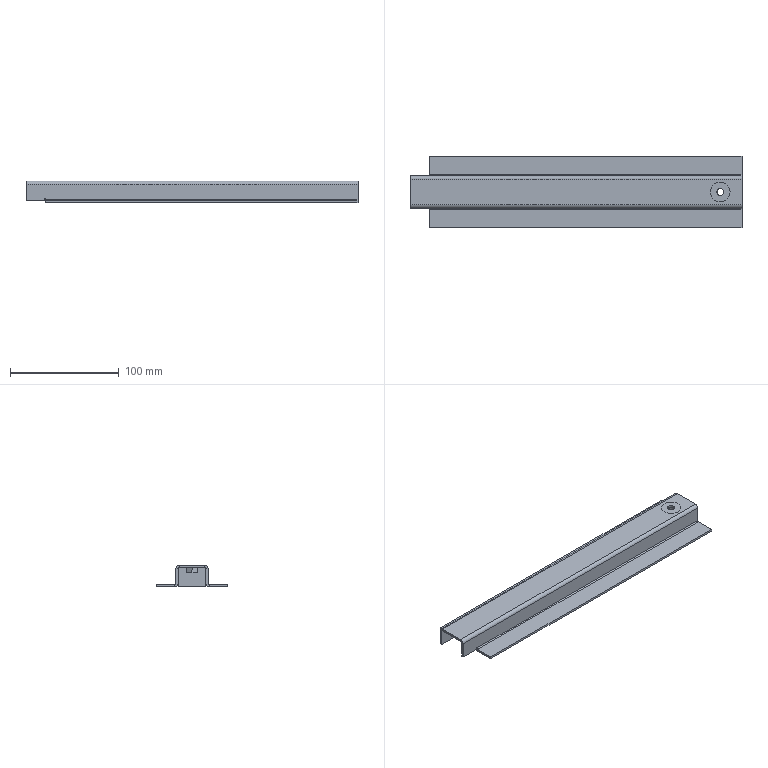Part | SolidWorks | features BaseBody 2 | 2 solids | 69 faces | box 304.9 x 65.5 x 20 mm | volume 59555 mm3 | plane 53 | cylinder 16 | commonest cylinder face diameters 2 x6 6 x6 6.5 x2 18 x2